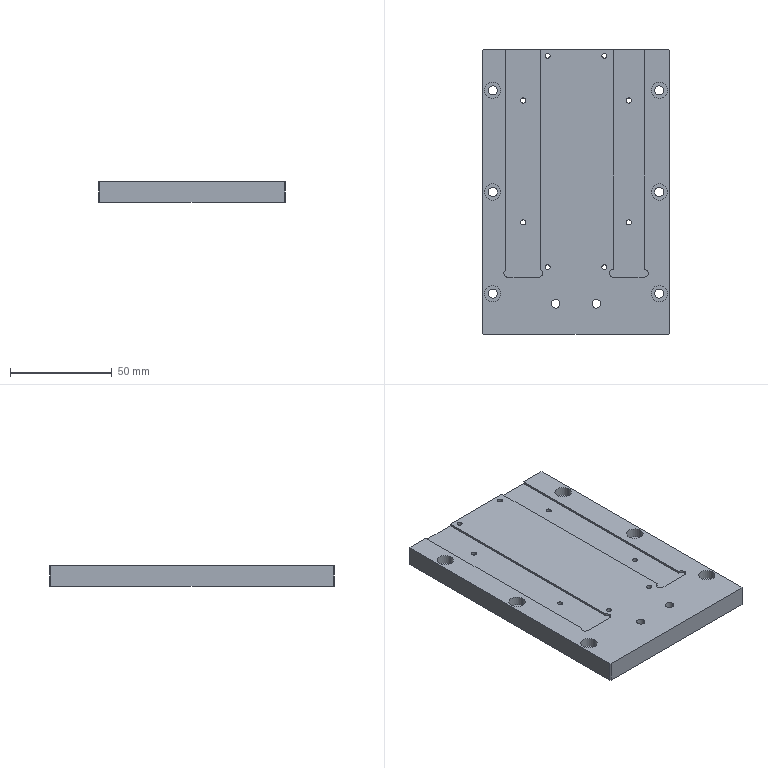Part | STEP file | 2026 Blade mounting base plate A | 1 solid | 74 faces | box 92 x 140 x 10 mm | volume 122641 mm3 | cylinder 50 | plane 24 | commonest cylinder face diameters 2.5 x16 4.5 x12 8 x12 4 x6 4.2 x4